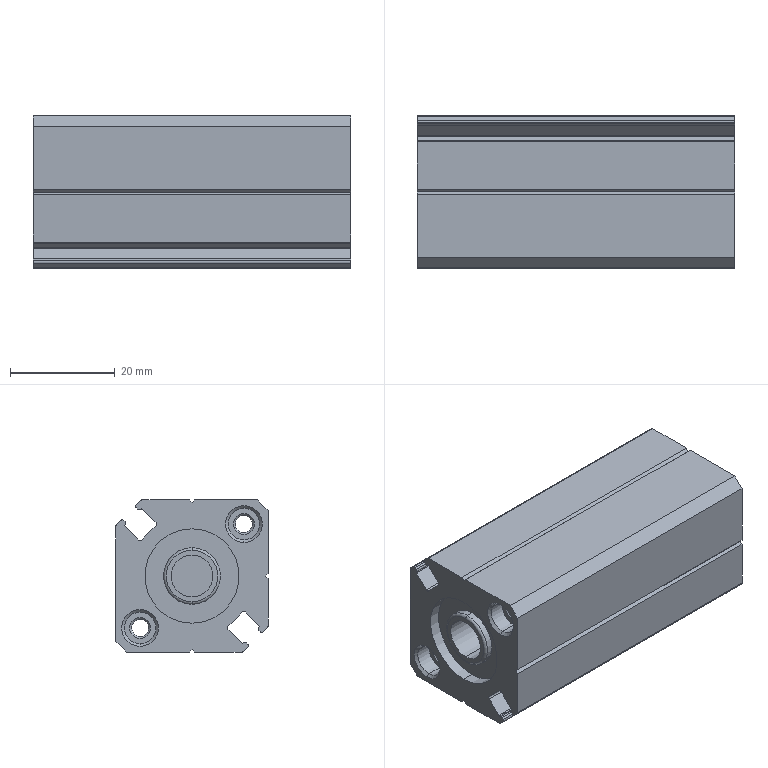Part | STEP file | 001-006-ACQS_16x3030_b | 1 solid | 111 faces | box 60.5 x 29 x 29 mm | volume 34569 mm3 | cylinder 48 | plane 41 | cone 20 | torus 2 | commonest cylinder face diameters 0.8 x19 6 x8 0.4 x5 3.242 x4 4.134 x4 8 x2